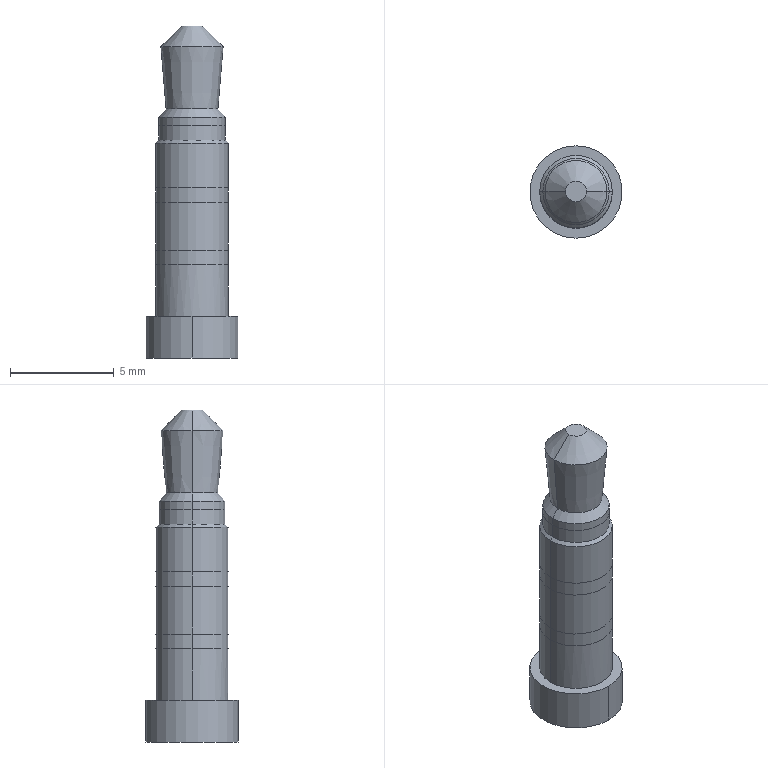Part | Creo | 1 solid | 27 faces | box 4.45 x 4.45 x 16 mm | volume 145.448 mm3 | cylinder 16 | cone 8 | plane 3 | commonest cylinder face diameters 3.5 x10 3.2 x4 4.45 x2
STEP:
#1=CARTESIAN_POINT('',(0.,0.,0.));
#2=DIRECTION('',(0.,0.,1.));
#3=DIRECTION('',(1.,0.,0.));
#4=AXIS2_PLACEMENT_3D('',#1,#2,#3);
#5=CARTESIAN_POINT('',(0.,0.075,-16.));
#6=VERTEX_POINT('',#5);
#7=CARTESIAN_POINT('',(0.,4.525,-16.));
#8=VERTEX_POINT('',#7);
#9=CARTESIAN_POINT('',(0.,2.3,-16.));
#10=DIRECTION('',(0.,0.,1.));
#11=DIRECTION('',(0.,-1.,0.));
#12=AXIS2_PLACEMENT_3D('',#9,#10,#11);
#13=CIRCLE('',#12,2.225);
#14=EDGE_CURVE('',#6,#8,#13,.T.);
#15=ORIENTED_EDGE('',*,*,#14,.F.);
#16=CARTESIAN_POINT('',(0.,0.075,-14.));
#17=VERTEX_POINT('',#16);
#18=CARTESIAN_POINT('',(0.,0.075,-16.));
#19=DIRECTION('',(0.,0.,1.));
#20=VECTOR('',#19,2.);
#21=LINE('',#18,#20);
#22=EDGE_CURVE('',#6,#17,#21,.T.);
#23=ORIENTED_EDGE('',*,*,#22,.T.);
#24=CARTESIAN_POINT('',(0.,4.525,-14.));
#25=VERTEX_POINT('',#24);
#26=CARTESIAN_POINT('',(0.,2.3,-14.));
#27=DIRECTION('',(0.,0.,-1.));
#28=DIRECTION('',(0.,1.,0.));
#29=AXIS2_PLACEMENT_3D('',#26,#27,#28);
#30=CIRCLE('',#29,2.225);
#31=EDGE_CURVE('',#25,#17,#30,.T.);
#32=ORIENTED_EDGE('',*,*,#31,.F.);
#33=CARTESIAN_POINT('',(0.,4.525,-16.));
#34=DIRECTION('',(0.,0.,1.));
#35=VECTOR('',#34,2.);
#36=LINE('',#33,#35);
#37=EDGE_CURVE('',#8,#25,#36,.T.);
#38=ORIENTED_EDGE('',*,*,#37,.F.);
#39=EDGE_LOOP('',(#15,#23,#32,#38));
#40=FACE_OUTER_BOUND('',#39,.F.);
#41=CARTESIAN_POINT('',(0.,2.3,-16.));
#42=DIRECTION('',(0.,0.,1.));
#43=DIRECTION('',(0.,-1.,0.));
#44=AXIS2_PLACEMENT_3D('',#41,#42,#43);
#45=CYLINDRICAL_SURFACE('',#44,2.225);
#46=ADVANCED_FACE('',(#40),#45,.T.);
#47=CARTESIAN_POINT('',(0.,2.3,-16.));
#48=DIRECTION('',(0.,0.,1.));
#49=DIRECTION('',(0.,1.,0.));
#50=AXIS2_PLACEMENT_3D('',#47,#48,#49);
#51=CIRCLE('',#50,2.225);
#52=EDGE_CURVE('',#8,#6,#51,.T.);
#53=ORIENTED_EDGE('',*,*,#52,.T.);
#54=ORIENTED_EDGE('',*,*,#14,.T.);
#55=EDGE_LOOP('',(#53,#54));
#56=FACE_OUTER_BOUND('',#55,.F.);
#57=CARTESIAN_POINT('',(0.,2.3,-16.));
#58=DIRECTION('',(0.,0.,-1.));
#59=DIRECTION('',(0.,1.,0.));
#60=AXIS2_PLACEMENT_3D('',#57,#58,#59);
#61=PLANE('',#60);
#62=ADVANCED_FACE('',(#56),#61,.T.);
#63=ORIENTED_EDGE('',*,*,#37,.T.);
#64=CARTESIAN_POINT('',(0.,2.3,-14.));
#65=DIRECTION('',(0.,0.,-1.));
#66=DIRECTION('',(0.,-1.,0.));
#67=AXIS2_PLACEMENT_3D('',#64,#65,#66);
#68=CIRCLE('',#67,2.225);
#69=EDGE_CURVE('',#17,#25,#68,.T.);
#70=ORIENTED_EDGE('',*,*,#69,.F.);
#71=ORIENTED_EDGE('',*,*,#22,.F.);
#72=ORIENTED_EDGE('',*,*,#52,.F.);
#73=EDGE_LOOP('',(#63,#70,#71,#72));
#74=FACE_OUTER_BOUND('',#73,.F.);
#75=CARTESIAN_POINT('',(0.,2.3,-16.));
#76=DIRECTION('',(0.,0.,1.));
#77=DIRECTION('',(0.,-1.,0.));
#78=AXIS2_PLACEMENT_3D('',#75,#76,#77);
#79=CYLINDRICAL_SURFACE('',#78,2.225);
#80=ADVANCED_FACE('',(#74),#79,.T.);
#81=ORIENTED_EDGE('',*,*,#69,.T.);
#82=ORIENTED_EDGE('',*,*,#31,.T.);
#83=EDGE_LOOP('',(#81,#82));
#84=FACE_OUTER_BOUND('',#83,.F.);
#85=CARTESIAN_POINT('',(0.,0.55,-14.));
#86=VERTEX_POINT('',#85);
#87=CARTESIAN_POINT('',(1.75,2.3,-14.));
#88=VERTEX_POINT('',#87);
#89=CARTESIAN_POINT('',(0.,2.3,-14.));
#90=DIRECTION('',(0.,0.,1.));
#91=DIRECTION('',(0.,-1.,0.));
#92=AXIS2_PLACEMENT_3D('',#89,#90,#91);
#93=CIRCLE('',#92,1.75);
#94=EDGE_CURVE('',#86,#88,#93,.T.);
#95=ORIENTED_EDGE('',*,*,#94,.T.);
#96=CARTESIAN_POINT('',(-1.75,2.3,-14.));
#97=VERTEX_POINT('',#96);
#98=CARTESIAN_POINT('',(0.,2.3,-14.));
#99=DIRECTION('',(0.,0.,1.));
#100=DIRECTION('',(1.,0.,0.));
#101=AXIS2_PLACEMENT_3D('',#98,#99,#100);
#102=CIRCLE('',#101,1.75);
#103=EDGE_CURVE('',#88,#97,#102,.T.);
#104=ORIENTED_EDGE('',*,*,#103,.T.);
#105=CARTESIAN_POINT('',(0.,2.3,-14.));
#106=DIRECTION('',(0.,0.,1.));
#107=DIRECTION('',(-1.,0.,0.));
#108=AXIS2_PLACEMENT_3D('',#105,#106,#107);
#109=CIRCLE('',#108,1.75);
#110=EDGE_CURVE('',#97,#86,#109,.T.);
#111=ORIENTED_EDGE('',*,*,#110,.T.);
#112=EDGE_LOOP('',(#95,#104,#111));
#113=FACE_BOUND('',#112,.F.);
#114=CARTESIAN_POINT('',(0.,2.3,-14.));
#115=DIRECTION('',(0.,0.,-1.));
#116=DIRECTION('',(0.,1.,0.));
#117=AXIS2_PLACEMENT_3D('',#114,#115,#116);
#118=PLANE('',#117);
#119=ADVANCED_FACE('',(#84,#113),#118,.F.);
#120=CARTESIAN_POINT('',(-1.75,2.3,-11.5));
#121=VERTEX_POINT('',#120);
#122=CARTESIAN_POINT('',(-1.75,2.3,-14.));
#123=DIRECTION('',(0.,0.,1.));
#124=VECTOR('',#123,2.5);
#125=LINE('',#122,#124);
#126=EDGE_CURVE('',#97,#121,#125,.T.);
#127=ORIENTED_EDGE('',*,*,#126,.T.);
#128=CARTESIAN_POINT('',(1.75,2.3,-11.5));
#129=VERTEX_POINT('',#128);
#130=CARTESIAN_POINT('',(0.,2.3,-11.5));
#131=DIRECTION('',(0.,0.,-1.));
#132=DIRECTION('',(1.,0.,0.));
#133=AXIS2_PLACEMENT_3D('',#130,#131,#132);
#134=CIRCLE('',#133,1.75);
#135=EDGE_CURVE('',#129,#121,#134,.T.);
#136=ORIENTED_EDGE('',*,*,#135,.F.);
#137=CARTESIAN_POINT('',(1.75,2.3,-14.));
#138=DIRECTION('',(0.,0.,1.));
#139=VECTOR('',#138,2.5);
#140=LINE('',#137,#139);
#141=EDGE_CURVE('',#88,#129,#140,.T.);
#142=ORIENTED_EDGE('',*,*,#141,.F.);
#143=ORIENTED_EDGE('',*,*,#94,.F.);
#144=ORIENTED_EDGE('',*,*,#110,.F.);
#145=EDGE_LOOP('',(#127,#136,#142,#143,#144));
#146=FACE_OUTER_BOUND('',#145,.F.);
#147=CARTESIAN_POINT('',(0.,2.3,0.));
#148=DIRECTION('',(0.,0.,1.));
#149=DIRECTION('',(1.,0.,0.));
#150=AXIS2_PLACEMENT_3D('',#147,#148,#149);
#151=CYLINDRICAL_SURFACE('',#150,1.75);
#152=ADVANCED_FACE('',(#146),#151,.T.);
#153=ORIENTED_EDGE('',*,*,#103,.F.);
#154=ORIENTED_EDGE('',*,*,#141,.T.);
#155=CARTESIAN_POINT('',(0.,2.3,-11.5));
#156=DIRECTION('',(0.,0.,-1.));
#157=DIRECTION('',(-1.,0.,0.));
#158=AXIS2_PLACEMENT_3D('',#155,#156,#157);
#159=CIRCLE('',#158,1.75);
#160=EDGE_CURVE('',#121,#129,#159,.T.);
#161=ORIENTED_EDGE('',*,*,#160,.F.);
#162=ORIENTED_EDGE('',*,*,#126,.F.);
#163=EDGE_LOOP('',(#153,#154,#161,#162));
#164=FACE_OUTER_BOUND('',#163,.F.);
#165=CARTESIAN_POINT('',(0.,2.3,0.));
#166=DIRECTION('',(0.,0.,1.));
#167=DIRECTION('',(1.,0.,0.));
#168=AXIS2_PLACEMENT_3D('',#165,#166,#167);
#169=CYLINDRICAL_SURFACE('',#168,1.75);
#170=ADVANCED_FACE('',(#164),#169,.T.);
#171=ORIENTED_EDGE('',*,*,#160,.T.);
#172=CARTESIAN_POINT('',(1.75,2.3,-10.8));
#173=VERTEX_POINT('',#172);
#174=CARTESIAN_POINT('',(1.75,2.3,-11.5));
#175=DIRECTION('',(0.,0.,1.));
#176=VECTOR('',#175,0.7);
#177=LINE('',#174,#176);
#178=EDGE_CURVE('',#129,#173,#177,.T.);
#179=ORIENTED_EDGE('',*,*,#178,.T.);
#180=CARTESIAN_POINT('',(-1.75,2.3,-10.8));
#181=VERTEX_POINT('',#180);
#182=CARTESIAN_POINT('',(0.,2.3,-10.8));
#183=DIRECTION('',(0.,0.,-1.));
#184=DIRECTION('',(-1.,0.,0.));
#185=AXIS2_PLACEMENT_3D('',#182,#183,#184);
#186=CIRCLE('',#185,1.75);
#187=EDGE_CURVE('',#181,#173,#186,.T.);
#188=ORIENTED_EDGE('',*,*,#187,.F.);
#189=CARTESIAN_POINT('',(-1.75,2.3,-11.5));
#190=DIRECTION('',(0.,0.,1.));
#191=VECTOR('',#190,0.7);
#192=LINE('',#189,#191);
#193=EDGE_CURVE('',#121,#181,#192,.T.);
#194=ORIENTED_EDGE('',*,*,#193,.F.);
#195=EDGE_LOOP('',(#171,#179,#188,#194));
#196=FACE_OUTER_BOUND('',#195,.F.);
#197=CARTESIAN_POINT('',(0.,2.3,0.));
#198=DIRECTION('',(0.,0.,1.));
#199=DIRECTION('',(1.,0.,0.));
#200=AXIS2_PLACEMENT_3D('',#197,#198,#199);
#201=CYLINDRICAL_SURFACE('',#200,1.75);
#202=ADVANCED_FACE('',(#196),#201,.T.);
#203=ORIENTED_EDGE('',*,*,#193,.T.);
#204=CARTESIAN_POINT('',(0.,2.3,-10.8));
#205=DIRECTION('',(0.,0.,-1.));
#206=DIRECTION('',(1.,0.,0.));
#207=AXIS2_PLACEMENT_3D('',#204,#205,#206);
#208=CIRCLE('',#207,1.75);
#209=EDGE_CURVE('',#173,#181,#208,.T.);
#210=ORIENTED_EDGE('',*,*,#209,.F.);
#211=ORIENTED_EDGE('',*,*,#178,.F.);
#212=ORIENTED_EDGE('',*,*,#135,.T.);
#213=EDGE_LOOP('',(#203,#210,#211,#212));
#214=FACE_OUTER_BOUND('',#213,.F.);
#215=CARTESIAN_POINT('',(0.,2.3,0.));
#216=DIRECTION('',(0.,0.,1.));
#217=DIRECTION('',(1.,0.,0.));
#218=AXIS2_PLACEMENT_3D('',#215,#216,#217);
#219=CYLINDRICAL_SURFACE('',#218,1.75);
#220=ADVANCED_FACE('',(#214),#219,.T.);
#221=CARTESIAN_POINT('',(-1.75,2.3,-8.5));
#222=VERTEX_POINT('',#221);
#223=CARTESIAN_POINT('',(-1.75,2.3,-10.8));
#224=DIRECTION('',(0.,0.,1.));
#225=VECTOR('',#224,2.3);
#226=LINE('',#223,#225);
#227=EDGE_CURVE('',#181,#222,#226,.T.);
#228=ORIENTED_EDGE('',*,*,#227,.T.);
#229=CARTESIAN_POINT('',(1.75,2.3,-8.5));
#230=VERTEX_POINT('',#229);
#231=CARTESIAN_POINT('',(0.,2.3,-8.5));
#232=DIRECTION('',(0.,0.,-1.));
#233=DIRECTION('',(1.,0.,0.));
#234=AXIS2_PLACEMENT_3D('',#231,#232,#233);
#235=CIRCLE('',#234,1.75);
#236=EDGE_CURVE('',#230,#222,#235,.T.);
#237=ORIENTED_EDGE('',*,*,#236,.F.);
#238=CARTESIAN_POINT('',(1.75,2.3,-10.8));
#239=DIRECTION('',(0.,0.,1.));
#240=VECTOR('',#239,2.3);
#241=LINE('',#238,#240);
#242=EDGE_CURVE('',#173,#230,#241,.T.);
#243=ORIENTED_EDGE('',*,*,#242,.F.);
#244=ORIENTED_EDGE('',*,*,#209,.T.);
#245=EDGE_LOOP('',(#228,#237,#243,#244));
#246=FACE_OUTER_BOUND('',#245,.F.);
#247=CARTESIAN_POINT('',(0.,2.3,0.));
#248=DIRECTION('',(0.,0.,1.));
#249=DIRECTION('',(1.,0.,0.));
#250=AXIS2_PLACEMENT_3D('',#247,#248,#249);
#251=CYLINDRICAL_SURFACE('',#250,1.75);
#252=ADVANCED_FACE('',(#246),#251,.T.);
#253=ORIENTED_EDGE('',*,*,#187,.T.);
#254=ORIENTED_EDGE('',*,*,#242,.T.);
#255=CARTESIAN_POINT('',(0.,2.3,-8.5));
#256=DIRECTION('',(0.,0.,-1.));
#257=DIRECTION('',(-1.,0.,0.));
#258=AXIS2_PLACEMENT_3D('',#255,#256,#257);
#259=CIRCLE('',#258,1.75);
#260=EDGE_CURVE('',#222,#230,#259,.T.);
#261=ORIENTED_EDGE('',*,*,#260,.F.);
#262=ORIENTED_EDGE('',*,*,#227,.F.);
#263=EDGE_LOOP('',(#253,#254,#261,#262));
#264=FACE_OUTER_BOUND('',#263,.F.);
#265=CARTESIAN_POINT('',(0.,2.3,0.));
#266=DIRECTION('',(0.,0.,1.));
#267=DIRECTION('',(1.,0.,0.));
#268=AXIS2_PLACEMENT_3D('',#265,#266,#267);
#269=CYLINDRICAL_SURFACE('',#268,1.75);
#270=ADVANCED_FACE('',(#264),#269,.T.);
#271=ORIENTED_EDGE('',*,*,#260,.T.);
#272=CARTESIAN_POINT('',(1.75,2.3,-7.8));
#273=VERTEX_POINT('',#272);
#274=CARTESIAN_POINT('',(1.75,2.3,-8.5));
#275=DIRECTION('',(0.,0.,1.));
#276=VECTOR('',#275,0.7);
#277=LINE('',#274,#276);
#278=EDGE_CURVE('',#230,#273,#277,.T.);
#279=ORIENTED_EDGE('',*,*,#278,.T.);
#280=CARTESIAN_POINT('',(-1.75,2.3,-7.8));
#281=VERTEX_POINT('',#280);
#282=CARTESIAN_POINT('',(0.,2.3,-7.8));
#283=DIRECTION('',(0.,0.,-1.));
#284=DIRECTION('',(-1.,0.,0.));
#285=AXIS2_PLACEMENT_3D('',#282,#283,#284);
#286=CIRCLE('',#285,1.75);
#287=EDGE_CURVE('',#281,#273,#286,.T.);
#288=ORIENTED_EDGE('',*,*,#287,.F.);
#289=CARTESIAN_POINT('',(-1.75,2.3,-8.5));
#290=DIRECTION('',(0.,0.,1.));
#291=VECTOR('',#290,0.7);
#292=LINE('',#289,#291);
#293=EDGE_CURVE('',#222,#281,#292,.T.);
#294=ORIENTED_EDGE('',*,*,#293,.F.);
#295=EDGE_LOOP('',(#271,#279,#288,#294));
#296=FACE_OUTER_BOUND('',#295,.F.);
#297=CARTESIAN_POINT('',(0.,2.3,0.));
#298=DIRECTION('',(0.,0.,1.));
#299=DIRECTION('',(1.,0.,0.));
#300=AXIS2_PLACEMENT_3D('',#297,#298,#299);
#301=CYLINDRICAL_SURFACE('',#300,1.75);
#302=ADVANCED_FACE('',(#296),#301,.T.);
#303=ORIENTED_EDGE('',*,*,#293,.T.);
#304=CARTESIAN_POINT('',(0.,2.3,-7.8));
#305=DIRECTION('',(0.,0.,-1.));
#306=DIRECTION('',(1.,0.,0.));
#307=AXIS2_PLACEMENT_3D('',#304,#305,#306);
#308=CIRCLE('',#307,1.75);
#309=EDGE_CURVE('',#273,#281,#308,.T.);
#310=ORIENTED_EDGE('',*,*,#309,.F.);
#311=ORIENTED_EDGE('',*,*,#278,.F.);
#312=ORIENTED_EDGE('',*,*,#236,.T.);
#313=EDGE_LOOP('',(#303,#310,#311,#312));
#314=FACE_OUTER_BOUND('',#313,.F.);
#315=CARTESIAN_POINT('',(0.,2.3,0.));
#316=DIRECTION('',(0.,0.,1.));
#317=DIRECTION('',(1.,0.,0.));
#318=AXIS2_PLACEMENT_3D('',#315,#316,#317);
#319=CYLINDRICAL_SURFACE('',#318,1.75);
#320=ADVANCED_FACE('',(#314),#319,.T.);
#321=CARTESIAN_POINT('',(-1.75,2.3,-5.65));
#322=VERTEX_POINT('',#321);
#323=CARTESIAN_POINT('',(-1.75,2.3,-7.8));
#324=DIRECTION('',(0.,0.,1.));
#325=VECTOR('',#324,2.15);
#326=LINE('',#323,#325);
#327=EDGE_CURVE('',#281,#322,#326,.T.);
#328=ORIENTED_EDGE('',*,*,#327,.T.);
#329=CARTESIAN_POINT('',(1.75,2.3,-5.65));
#330=VERTEX_POINT('',#329);
#331=CARTESIAN_POINT('',(0.,2.3,-5.65));
#332=DIRECTION('',(0.,0.,-1.));
#333=DIRECTION('',(1.,0.,0.));
#334=AXIS2_PLACEMENT_3D('',#331,#332,#333);
#335=CIRCLE('',#334,1.75);
#336=EDGE_CURVE('',#330,#322,#335,.T.);
#337=ORIENTED_EDGE('',*,*,#336,.F.);
#338=CARTESIAN_POINT('',(1.75,2.3,-7.8));
#339=DIRECTION('',(0.,0.,1.));
#340=VECTOR('',#339,2.15);
#341=LINE('',#338,#340);
#342=EDGE_CURVE('',#273,#330,#341,.T.);
#343=ORIENTED_EDGE('',*,*,#342,.F.);
#344=ORIENTED_EDGE('',*,*,#309,.T.);
#345=EDGE_LOOP('',(#328,#337,#343,#344));
#346=FACE_OUTER_BOUND('',#345,.F.);
#347=CARTESIAN_POINT('',(0.,2.3,0.));
#348=DIRECTION('',(0.,0.,1.));
#349=DIRECTION('',(1.,0.,0.));
#350=AXIS2_PLACEMENT_3D('',#347,#348,#349);
#351=CYLINDRICAL_SURFACE('',#350,1.75);
#352=ADVANCED_FACE('',(#346),#351,.T.);
#353=ORIENTED_EDGE('',*,*,#287,.T.);
#354=ORIENTED_EDGE('',*,*,#342,.T.);
#355=CARTESIAN_POINT('',(0.,2.3,-5.65));
#356=DIRECTION('',(0.,0.,-1.));
#357=DIRECTION('',(-1.,0.,0.));
#358=AXIS2_PLACEMENT_3D('',#355,#356,#357);
#359=CIRCLE('',#358,1.75);
#360=EDGE_CURVE('',#322,#330,#359,.T.);
#361=ORIENTED_EDGE('',*,*,#360,.F.);
#362=ORIENTED_EDGE('',*,*,#327,.F.);
#363=EDGE_LOOP('',(#353,#354,#361,#362));
#364=FACE_OUTER_BOUND('',#363,.F.);
#365=CARTESIAN_POINT('',(0.,2.3,0.));
#366=DIRECTION('',(0.,0.,1.));
#367=DIRECTION('',(1.,0.,0.));
#368=AXIS2_PLACEMENT_3D('',#365,#366,#367);
#369=CYLINDRICAL_SURFACE('',#368,1.75);
#370=ADVANCED_FACE('',(#364),#369,.T.);
#371=CARTESIAN_POINT('',(1.6,2.3,-5.5));
#372=VERTEX_POINT('',#371);
#373=CARTESIAN_POINT('',(-1.6,2.3,-5.5));
#374=VERTEX_POINT('',#373);
#375=CARTESIAN_POINT('',(0.,2.3,-5.5));
#376=DIRECTION('',(0.,0.,1.));
#377=DIRECTION('',(1.,0.,0.));
#378=AXIS2_PLACEMENT_3D('',#375,#376,#377);
#379=CIRCLE('',#378,1.6);
#380=EDGE_CURVE('',#372,#374,#379,.T.);
#381=ORIENTED_EDGE('',*,*,#380,.T.);
#382=CARTESIAN_POINT('',(-1.6,2.3,-5.5));
#383=DIRECTION('',(-0.7071,0.,-0.7071));
#384=VECTOR('',#383,0.2121);
#385=LINE('',#382,#384);
#386=EDGE_CURVE('',#374,#322,#385,.T.);
#387=ORIENTED_EDGE('',*,*,#386,.T.);
#388=ORIENTED_EDGE('',*,*,#360,.T.);
#389=CARTESIAN_POINT('',(1.6,2.3,-5.5));
#390=DIRECTION('',(0.7071,0.,-0.7071));
#391=VECTOR('',#390,0.2121);
#392=LINE('',#389,#391);
#393=EDGE_CURVE('',#372,#330,#392,.T.);
#394=ORIENTED_EDGE('',*,*,#393,.F.);
#395=EDGE_LOOP('',(#381,#387,#388,#394));
#396=FACE_OUTER_BOUND('',#395,.F.);
#397=CARTESIAN_POINT('',(0.,2.3,-5.575));
#398=DIRECTION('',(0.,0.,-1.));
#399=DIRECTION('',(-1.,0.,0.));
#400=AXIS2_PLACEMENT_3D('',#397,#398,#399);
#401=CONICAL_SURFACE('',#400,1.675,45.);
#402=ADVANCED_FACE('',(#396),#401,.T.);
#403=ORIENTED_EDGE('',*,*,#380,.F.);
#404=CARTESIAN_POINT('',(1.6,2.3,-4.8));
#405=VERTEX_POINT('',#404);
#406=CARTESIAN_POINT('',(1.6,2.3,-5.5));
#407=DIRECTION('',(0.,0.,1.));
#408=VECTOR('',#407,0.7);
#409=LINE('',#406,#408);
#410=EDGE_CURVE('',#372,#405,#409,.T.);
#411=ORIENTED_EDGE('',*,*,#410,.T.);
#412=CARTESIAN_POINT('',(-1.6,2.3,-4.8));
#413=VERTEX_POINT('',#412);
#414=CARTESIAN_POINT('',(0.,2.3,-4.8));
#415=DIRECTION('',(0.,0.,1.));
#416=DIRECTION('',(1.,0.,0.));
#417=AXIS2_PLACEMENT_3D('',#414,#415,#416);
#418=CIRCLE('',#417,1.6);
#419=EDGE_CURVE('',#405,#413,#418,.T.);
#420=ORIENTED_EDGE('',*,*,#419,.T.);
#421=CARTESIAN_POINT('',(-1.6,2.3,-5.5));
#422=DIRECTION('',(0.,0.,1.));
#423=VECTOR('',#422,0.7);
#424=LINE('',#421,#423);
#425=EDGE_CURVE('',#374,#413,#424,.T.);
#426=ORIENTED_EDGE('',*,*,#425,.F.);
#427=EDGE_LOOP('',(#403,#411,#420,#426));
#428=FACE_OUTER_BOUND('',#427,.F.);
#429=CARTESIAN_POINT('',(0.,2.3,0.));
#430=DIRECTION('',(0.,0.,1.));
#431=DIRECTION('',(1.,0.,0.));
#432=AXIS2_PLACEMENT_3D('',#429,#430,#431);
#433=CYLINDRICAL_SURFACE('',#432,1.6);
#434=ADVANCED_FACE('',(#428),#433,.T.);
#435=ORIENTED_EDGE('',*,*,#425,.T.);
#436=CARTESIAN_POINT('',(0.,2.3,-4.8));
#437=DIRECTION('',(0.,0.,1.));
#438=DIRECTION('',(-1.,0.,0.));
#439=AXIS2_PLACEMENT_3D('',#436,#437,#438);
#440=CIRCLE('',#439,1.6);
#441=EDGE_CURVE('',#413,#405,#440,.T.);
#442=ORIENTED_EDGE('',*,*,#441,.T.);
#443=ORIENTED_EDGE('',*,*,#410,.F.);
#444=CARTESIAN_POINT('',(0.,2.3,-5.5));
#445=DIRECTION('',(0.,0.,1.));
#446=DIRECTION('',(-1.,0.,0.));
#447=AXIS2_PLACEMENT_3D('',#444,#445,#446);
#448=CIRCLE('',#447,1.6);
#449=EDGE_CURVE('',#374,#372,#448,.T.);
#450=ORIENTED_EDGE('',*,*,#449,.F.);
#451=EDGE_LOOP('',(#435,#442,#443,#450));
#452=FACE_OUTER_BOUND('',#451,.F.);
#453=CARTESIAN_POINT('',(0.,2.3,0.));
#454=DIRECTION('',(0.,0.,1.));
#455=DIRECTION('',(1.,0.,0.));
#456=AXIS2_PLACEMENT_3D('',#453,#454,#455);
#457=CYLINDRICAL_SURFACE('',#456,1.6);
#458=ADVANCED_FACE('',(#452),#457,.T.);
#459=CARTESIAN_POINT('',(-1.6,2.3,-4.4));
#460=VERTEX_POINT('',#459);
#461=CARTESIAN_POINT('',(-1.6,2.3,-4.8));
#462=DIRECTION('',(0.,0.,1.));
#463=VECTOR('',#462,0.4);
#464=LINE('',#461,#463);
#465=EDGE_CURVE('',#413,#460,#464,.T.);
#466=ORIENTED_EDGE('',*,*,#465,.T.);
#467=CARTESIAN_POINT('',(1.6,2.3,-4.4));
#468=VERTEX_POINT('',#467);
#469=CARTESIAN_POINT('',(0.,2.3,-4.4));
#470=DIRECTION('',(0.,0.,-1.));
#471=DIRECTION('',(1.,0.,0.));
#472=AXIS2_PLACEMENT_3D('',#469,#470,#471);
#473=CIRCLE('',#472,1.6);
#474=EDGE_CURVE('',#468,#460,#473,.T.);
#475=ORIENTED_EDGE('',*,*,#474,.F.);
#476=CARTESIAN_POINT('',(1.6,2.3,-4.8));
#477=DIRECTION('',(0.,0.,1.));
#478=VECTOR('',#477,0.4);
#479=LINE('',#476,#478);
#480=EDGE_CURVE('',#405,#468,#479,.T.);
#481=ORIENTED_EDGE('',*,*,#480,.F.);
#482=ORIENTED_EDGE('',*,*,#441,.F.);
#483=EDGE_LOOP('',(#466,#475,#481,#482));
#484=FACE_OUTER_BOUND('',#483,.F.);
#485=CARTESIAN_POINT('',(0.,2.3,0.));
#486=DIRECTION('',(0.,0.,1.));
#487=DIRECTION('',(1.,0.,0.));
#488=AXIS2_PLACEMENT_3D('',#485,#486,#487);
#489=CYLINDRICAL_SURFACE('',#488,1.6);
#490=ADVANCED_FACE('',(#484),#489,.T.);
#491=ORIENTED_EDGE('',*,*,#419,.F.);
#492=ORIENTED_EDGE('',*,*,#480,.T.);
#493=CARTESIAN_POINT('',(0.,2.3,-4.4));
#494=DIRECTION('',(0.,0.,-1.));
#495=DIRECTION('',(-1.,0.,0.));
#496=AXIS2_PLACEMENT_3D('',#493,#494,#495);
#497=CIRCLE('',#496,1.6);
#498=EDGE_CURVE('',#460,#468,#497,.T.);
#499=ORIENTED_EDGE('',*,*,#498,.F.);
#500=ORIENTED_EDGE('',*,*,#465,.F.);
#501=EDGE_LOOP('',(#491,#492,#499,#500));
#502=FACE_OUTER_BOUND('',#501,.F.);
#503=CARTESIAN_POINT('',(0.,2.3,0.));
#504=DIRECTION('',(0.,0.,1.));
#505=DIRECTION('',(1.,0.,0.));
#506=AXIS2_PLACEMENT_3D('',#503,#504,#505);
#507=CYLINDRICAL_SURFACE('',#506,1.6);
#508=ADVANCED_FACE('',(#502),#507,.T.);
#509=CARTESIAN_POINT('',(1.25,2.3,-4.));
#510=VERTEX_POINT('',#509);
#511=CARTESIAN_POINT('',(-1.25,2.3,-4.));
#512=VERTEX_POINT('',#511);
#513=CARTESIAN_POINT('',(0.,2.3,-4.));
#514=DIRECTION('',(0.,0.,1.));
#515=DIRECTION('',(1.,0.,0.));
#516=AXIS2_PLACEMENT_3D('',#513,#514,#515);
#517=CIRCLE('',#516,1.25);
#518=EDGE_CURVE('',#510,#512,#517,.T.);
#519=ORIENTED_EDGE('',*,*,#518,.T.);
#520=CARTESIAN_POINT('',(-1.25,2.3,-4.));
#521=DIRECTION('',(-0.6585,0.,-0.7526));
#522=VECTOR('',#521,0.5315);
#523=LINE('',#520,#522);
#524=EDGE_CURVE('',#512,#460,#523,.T.);
#525=ORIENTED_EDGE('',*,*,#524,.T.);
#526=ORIENTED_EDGE('',*,*,#498,.T.);
#527=CARTESIAN_POINT('',(1.25,2.3,-4.));
#528=DIRECTION('',(0.6585,0.,-0.7526));
#529=VECTOR('',#528,0.5315);
#530=LINE('',#527,#529);
#531=EDGE_CURVE('',#510,#468,#530,.T.);
#532=ORIENTED_EDGE('',*,*,#531,.F.);
#533=EDGE_LOOP('',(#519,#525,#526,#532));
#534=FACE_OUTER_BOUND('',#533,.F.);
#535=CARTESIAN_POINT('',(0.,2.3,-4.2));
#536=DIRECTION('',(0.,0.,-1.));
#537=DIRECTION('',(-1.,0.,0.));
#538=AXIS2_PLACEMENT_3D('',#535,#536,#537);
#539=CONICAL_SURFACE('',#538,1.425,41.186);
#540=ADVANCED_FACE('',(#534),#539,.T.);
#541=ORIENTED_EDGE('',*,*,#518,.F.);
#542=CARTESIAN_POINT('',(1.5,2.3,-1.));
#543=VERTEX_POINT('',#542);
#544=CARTESIAN_POINT('',(1.25,2.3,-4.));
#545=DIRECTION('',(0.08305,0.,0.9965));
#546=VECTOR('',#545,3.01);
#547=LINE('',#544,#546);
#548=EDGE_CURVE('',#510,#543,#547,.T.);
#549=ORIENTED_EDGE('',*,*,#548,.T.);
#550=CARTESIAN_POINT('',(-1.5,2.3,-1.));
#551=VERTEX_POINT('',#550);
#552=CARTESIAN_POINT('',(0.,2.3,-1.));
#553=DIRECTION('',(0.,0.,1.));
#554=DIRECTION('',(1.,0.,0.));
#555=AXIS2_PLACEMENT_3D('',#552,#553,#554);
#556=CIRCLE('',#555,1.5);
#557=EDGE_CURVE('',#543,#551,#556,.T.);
#558=ORIENTED_EDGE('',*,*,#557,.T.);
#559=CARTESIAN_POINT('',(-1.25,2.3,-4.));
#560=DIRECTION('',(-0.08305,0.,0.9965));
#561=VECTOR('',#560,3.01);
#562=LINE('',#559,#561);
#563=EDGE_CURVE('',#512,#551,#562,.T.);
#564=ORIENTED_EDGE('',*,*,#563,.F.);
#565=EDGE_LOOP('',(#541,#549,#558,#564));
#566=FACE_OUTER_BOUND('',#565,.F.);
#567=CARTESIAN_POINT('',(0.,2.3,-2.5));
#568=DIRECTION('',(0.,0.,1.));
#569=DIRECTION('',(1.,0.,0.));
#570=AXIS2_PLACEMENT_3D('',#567,#568,#569);
#571=CONICAL_SURFACE('',#570,1.375,4.764);
#572=ADVANCED_FACE('',(#566),#571,.T.);
#573=ORIENTED_EDGE('',*,*,#563,.T.);
#574=CARTESIAN_POINT('',(0.,2.3,-1.));
#575=DIRECTION('',(0.,0.,1.));
#576=DIRECTION('',(-1.,0.,0.));
#577=AXIS2_PLACEMENT_3D('',#574,#575,#576);
#578=CIRCLE('',#577,1.5);
#579=EDGE_CURVE('',#551,#543,#578,.T.);
#580=ORIENTED_EDGE('',*,*,#579,.T.);
#581=ORIENTED_EDGE('',*,*,#548,.F.);
#582=CARTESIAN_POINT('',(0.,2.3,-4.));
#583=DIRECTION('',(0.,0.,1.));
#584=DIRECTION('',(-1.,0.,0.));
#585=AXIS2_PLACEMENT_3D('',#582,#583,#584);
#586=CIRCLE('',#585,1.25);
#587=EDGE_CURVE('',#512,#510,#586,.T.);
#588=ORIENTED_EDGE('',*,*,#587,.F.);
#589=EDGE_LOOP('',(#573,#580,#581,#588));
#590=FACE_OUTER_BOUND('',#589,.F.);
#591=CARTESIAN_POINT('',(0.,2.3,-2.5));
#592=DIRECTION('',(0.,0.,1.));
#593=DIRECTION('',(1.,0.,0.));
#594=AXIS2_PLACEMENT_3D('',#591,#592,#593);
#595=CONICAL_SURFACE('',#594,1.375,4.764);
#596=ADVANCED_FACE('',(#590),#595,.T.);
#597=CARTESIAN_POINT('',(0.5,2.3,0.));
#598=VERTEX_POINT('',#597);
#599=CARTESIAN_POINT('',(0.5,2.3,0.));
#600=DIRECTION('',(0.7071,0.,-0.7071));
#601=VECTOR('',#600,1.414);
#602=LINE('',#599,#601);
#603=EDGE_CURVE('',#598,#543,#602,.T.);
#604=ORIENTED_EDGE('',*,*,#603,.T.);
#605=ORIENTED_EDGE('',*,*,#579,.F.);
#606=CARTESIAN_POINT('',(-0.5,2.3,0.));
#607=VERTEX_POINT('',#606);
#608=CARTESIAN_POINT('',(-0.5,2.3,0.));
#609=DIRECTION('',(-0.7071,0.,-0.7071));
#610=VECTOR('',#609,1.414);
#611=LINE('',#608,#610);
#612=EDGE_CURVE('',#607,#551,#611,.T.);
#613=ORIENTED_EDGE('',*,*,#612,.F.);
#614=CARTESIAN_POINT('',(0.,2.3,0.));
#615=DIRECTION('',(0.,0.,-1.));
#616=DIRECTION('',(1.,0.,0.));
#617=AXIS2_PLACEMENT_3D('',#614,#615,#616);
#618=CIRCLE('',#617,0.5);
#619=EDGE_CURVE('',#598,#607,#618,.T.);
#620=ORIENTED_EDGE('',*,*,#619,.F.);
#621=EDGE_LOOP('',(#604,#605,#613,#620));
#622=FACE_OUTER_BOUND('',#621,.F.);
#623=CARTESIAN_POINT('',(0.,2.3,-0.5));
#624=DIRECTION('',(0.,0.,-1.));
#625=DIRECTION('',(-1.,0.,0.));
#626=AXIS2_PLACEMENT_3D('',#623,#624,#625);
#627=CONICAL_SURFACE('',#626,1.,45.);
#628=ADVANCED_FACE('',(#622),#627,.T.);
#629=CARTESIAN_POINT('',(0.,2.3,0.));
#630=DIRECTION('',(0.,0.,-1.));
#631=DIRECTION('',(-1.,0.,0.));
#632=AXIS2_PLACEMENT_3D('',#629,#630,#631);
#633=CIRCLE('',#632,0.5);
#634=EDGE_CURVE('',#607,#598,#633,.T.);
#635=ORIENTED_EDGE('',*,*,#634,.F.);
#636=ORIENTED_EDGE('',*,*,#612,.T.);
#637=ORIENTED_EDGE('',*,*,#557,.F.);
#638=ORIENTED_EDGE('',*,*,#603,.F.);
#639=EDGE_LOOP('',(#635,#636,#637,#638));
#640=FACE_OUTER_BOUND('',#639,.F.);
#641=CARTESIAN_POINT('',(0.,2.3,-0.5));
#642=DIRECTION('',(0.,0.,-1.));
#643=DIRECTION('',(-1.,0.,0.));
#644=AXIS2_PLACEMENT_3D('',#641,#642,#643);
#645=CONICAL_SURFACE('',#644,1.,45.);
#646=ADVANCED_FACE('',(#640),#645,.T.);
#647=ORIENTED_EDGE('',*,*,#619,.T.);
#648=ORIENTED_EDGE('',*,*,#634,.T.);
#649=EDGE_LOOP('',(#647,#648));
#650=FACE_OUTER_BOUND('',#649,.F.);
#651=CARTESIAN_POINT('',(0.,2.3,0.));
#652=DIRECTION('',(0.,0.,-1.));
#653=DIRECTION('',(-1.,0.,0.));
#654=AXIS2_PLACEMENT_3D('',#651,#652,#653);
#655=PLANE('',#654);
#656=ADVANCED_FACE('',(#650),#655,.F.);
#657=ORIENTED_EDGE('',*,*,#531,.T.);
#658=ORIENTED_EDGE('',*,*,#474,.T.);
#659=ORIENTED_EDGE('',*,*,#524,.F.);
#660=ORIENTED_EDGE('',*,*,#587,.T.);
#661=EDGE_LOOP('',(#657,#658,#659,#660));
#662=FACE_OUTER_BOUND('',#661,.F.);
#663=CARTESIAN_POINT('',(0.,2.3,-4.2));
#664=DIRECTION('',(0.,0.,-1.));
#665=DIRECTION('',(-1.,0.,0.));
#666=AXIS2_PLACEMENT_3D('',#663,#664,#665);
#667=CONICAL_SURFACE('',#666,1.425,41.186);
#668=ADVANCED_FACE('',(#662),#667,.T.);
#669=ORIENTED_EDGE('',*,*,#393,.T.);
#670=ORIENTED_EDGE('',*,*,#336,.T.);
#671=ORIENTED_EDGE('',*,*,#386,.F.);
#672=ORIENTED_EDGE('',*,*,#449,.T.);
#673=EDGE_LOOP('',(#669,#670,#671,#672));
#674=FACE_OUTER_BOUND('',#673,.F.);
#675=CARTESIAN_POINT('',(0.,2.3,-5.575));
#676=DIRECTION('',(0.,0.,-1.));
#677=DIRECTION('',(-1.,0.,0.));
#678=AXIS2_PLACEMENT_3D('',#675,#676,#677);
#679=CONICAL_SURFACE('',#678,1.675,45.);
#680=ADVANCED_FACE('',(#674),#679,.T.);
#681=CLOSED_SHELL('',(#46,#62,#80,#119,#152,#170,#202,#220,#252,#270,#302,#320,#352,#370,#402,#434,#458,#490,#508,#540,#572,#596,#628,#646,#656,#668,#680));
#682=MANIFOLD_SOLID_BREP('',#681);
#683=(LENGTH_UNIT()NAMED_UNIT(*)SI_UNIT(.MILLI.,.METRE.));
#684=UNCERTAINTY_MEASURE_WITH_UNIT(LENGTH_MEASURE(0.001719),#683,'','');
#685=(NAMED_UNIT(*)PLANE_ANGLE_UNIT()SI_UNIT($,.RADIAN.));
#686=PLANE_ANGLE_MEASURE_WITH_UNIT(PLANE_ANGLE_MEASURE(0.01745),#685);
#687=(CONVERSION_BASED_UNIT('DEGREE',#686)NAMED_UNIT(*)PLANE_ANGLE_UNIT());
#688=(NAMED_UNIT(*)SI_UNIT($,.STERADIAN.)SOLID_ANGLE_UNIT());
#689=(GEOMETRIC_REPRESENTATION_CONTEXT(3)GLOBAL_UNCERTAINTY_ASSIGNED_CONTEXT((#684))GLOBAL_UNIT_ASSIGNED_CONTEXT((#683,#687,#688))REPRESENTATION_CONTEXT('',''));
#690=ADVANCED_BREP_SHAPE_REPRESENTATION('',(#4,#682),#689);